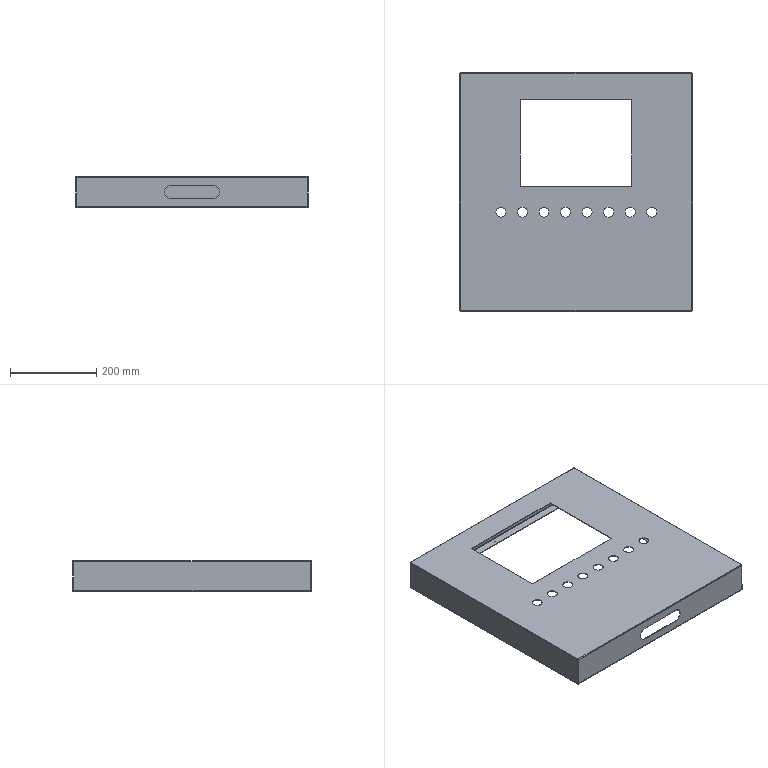Part | STEP file | x77-05101 | 1 solid | 110 faces | box 540 x 553 x 71.5 mm | volume 640844 mm3 | cylinder 50 | plane 44 | spline 16 | commonest cylinder face diameters 2.5 x16 23 x16 1.473 x8 4.473 x8 30 x2